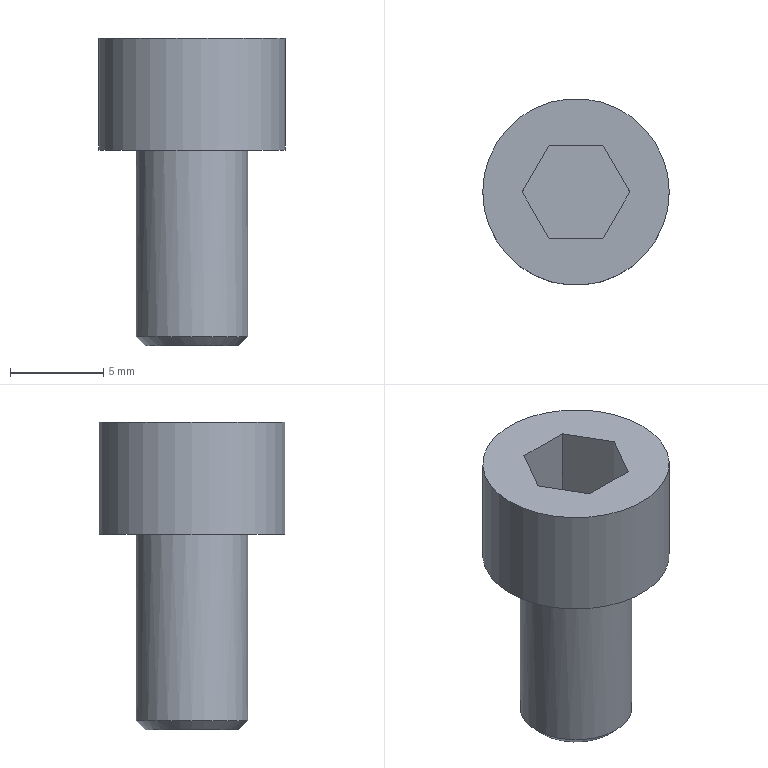Part | STEP file | solid 39 | 1 solid | 13 faces | box 10 x 10 x 16.5 mm | volume 680.158 mm3 | plane 10 | cylinder 2 | cone 1 | commonest cylinder face diameters 6 x1 10 x1